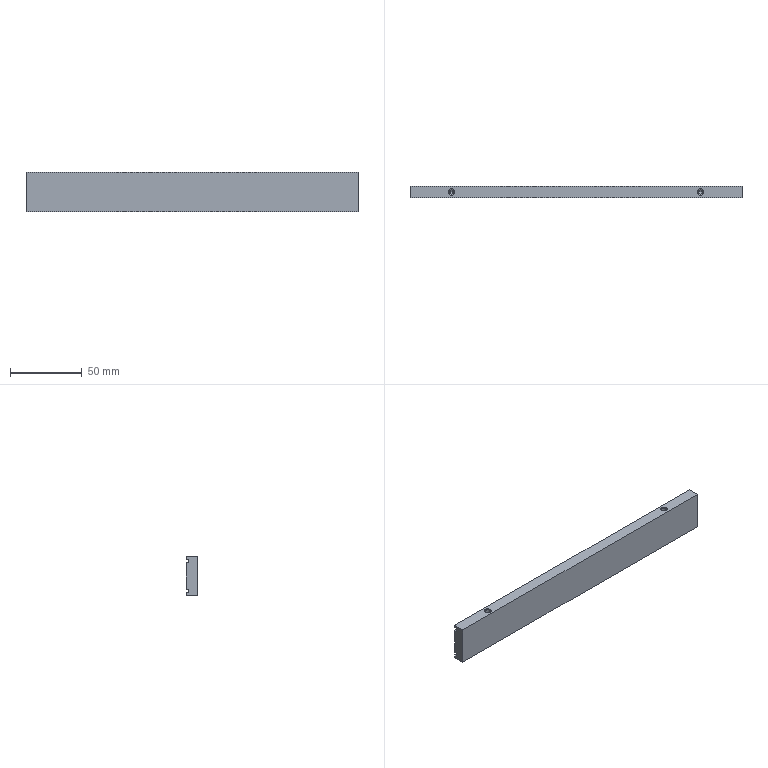Part | NX | 1 solid | 46 faces | box 232 x 8 x 27.6 mm | volume 49260 mm3 | cylinder 16 | cone 16 | plane 14 | commonest cylinder face diameters 3.3 x16
STEP:
#1=CARTESIAN_POINT('',(159.,209.7,-32.6));
#2=VERTEX_POINT('',#1);
#3=CARTESIAN_POINT('',(159.,208.2,-32.6));
#4=VERTEX_POINT('',#3);
#5=CARTESIAN_POINT('',(159.,0.,-32.6));
#6=DIRECTION('',(0.,-1.,0.));
#7=VECTOR('',#6,1000.);
#8=LINE('',#5,#7);
#9=EDGE_CURVE('',#2,#4,#8,.T.);
#10=ORIENTED_EDGE('',*,*,#9,.T.);
#11=CARTESIAN_POINT('',(391.,208.2,-32.6));
#12=VERTEX_POINT('',#11);
#13=CARTESIAN_POINT('',(0.,208.2,-32.6));
#14=DIRECTION('',(-1.,0.,0.));
#15=VECTOR('',#14,1000.);
#16=LINE('',#13,#15);
#17=EDGE_CURVE('',#12,#4,#16,.T.);
#18=ORIENTED_EDGE('',*,*,#17,.F.);
#19=CARTESIAN_POINT('',(391.,209.7,-32.6));
#20=VERTEX_POINT('',#19);
#21=CARTESIAN_POINT('',(391.,0.,-32.6));
#22=DIRECTION('',(0.,-1.,0.));
#23=VECTOR('',#22,1000.);
#24=LINE('',#21,#23);
#25=EDGE_CURVE('',#20,#12,#24,.T.);
#26=ORIENTED_EDGE('',*,*,#25,.F.);
#27=CARTESIAN_POINT('',(0.,209.7,-32.6));
#28=DIRECTION('',(1.,0.,0.));
#29=VECTOR('',#28,1000.);
#30=LINE('',#27,#29);
#31=EDGE_CURVE('',#2,#20,#30,.T.);
#32=ORIENTED_EDGE('',*,*,#31,.F.);
#33=EDGE_LOOP('',(#10,#18,#26,#32));
#34=FACE_BOUND('',#33,.T.);
#35=CARTESIAN_POINT('',(-62.051,211.112,-32.6));
#36=DIRECTION('',(0.,0.,-1.));
#37=DIRECTION('',(-1.,0.,0.));
#38=AXIS2_PLACEMENT_3D('',#35,#36,#37);
#39=PLANE('',#38);
#40=ADVANCED_FACE('',(#34),#39,.F.);
#41=CARTESIAN_POINT('',(159.,209.7,-51.4));
#42=VERTEX_POINT('',#41);
#43=CARTESIAN_POINT('',(159.,209.7,0.));
#44=DIRECTION('',(0.,0.,1.));
#45=VECTOR('',#44,1000.);
#46=LINE('',#43,#45);
#47=EDGE_CURVE('',#42,#2,#46,.T.);
#48=ORIENTED_EDGE('',*,*,#47,.T.);
#49=ORIENTED_EDGE('',*,*,#31,.T.);
#50=CARTESIAN_POINT('',(391.,209.7,-51.4));
#51=VERTEX_POINT('',#50);
#52=CARTESIAN_POINT('',(391.,209.7,0.));
#53=DIRECTION('',(0.,0.,-1.));
#54=VECTOR('',#53,1000.);
#55=LINE('',#52,#54);
#56=EDGE_CURVE('',#20,#51,#55,.T.);
#57=ORIENTED_EDGE('',*,*,#56,.T.);
#58=CARTESIAN_POINT('',(0.,209.7,-51.4));
#59=DIRECTION('',(-1.,0.,0.));
#60=VECTOR('',#59,1000.);
#61=LINE('',#58,#60);
#62=EDGE_CURVE('',#51,#42,#61,.T.);
#63=ORIENTED_EDGE('',*,*,#62,.T.);
#64=EDGE_LOOP('',(#48,#49,#57,#63));
#65=FACE_BOUND('',#64,.T.);
#66=CARTESIAN_POINT('',(652.949,209.7,-52.35));
#67=DIRECTION('',(0.,1.,0.));
#68=DIRECTION('',(1.,0.,0.));
#69=AXIS2_PLACEMENT_3D('',#66,#67,#68);
#70=PLANE('',#69);
#71=ADVANCED_FACE('',(#65),#70,.T.);
#72=ORIENTED_EDGE('',*,*,#47,.F.);
#73=CARTESIAN_POINT('',(159.,208.2,-51.4));
#74=VERTEX_POINT('',#73);
#75=CARTESIAN_POINT('',(159.,0.,-51.4));
#76=DIRECTION('',(0.,1.,0.));
#77=VECTOR('',#76,1000.);
#78=LINE('',#75,#77);
#79=EDGE_CURVE('',#74,#42,#78,.T.);
#80=ORIENTED_EDGE('',*,*,#79,.F.);
#81=CARTESIAN_POINT('',(159.,208.2,-53.6));
#82=VERTEX_POINT('',#81);
#83=CARTESIAN_POINT('',(159.,208.2,0.));
#84=DIRECTION('',(0.,0.,1.));
#85=VECTOR('',#84,1000.);
#86=LINE('',#83,#85);
#87=EDGE_CURVE('',#82,#74,#86,.T.);
#88=ORIENTED_EDGE('',*,*,#87,.F.);
#89=CARTESIAN_POINT('',(159.,209.7,-53.6));
#90=VERTEX_POINT('',#89);
#91=CARTESIAN_POINT('',(159.,0.,-53.6));
#92=DIRECTION('',(0.,-1.,0.));
#93=VECTOR('',#92,1000.);
#94=LINE('',#91,#93);
#95=EDGE_CURVE('',#90,#82,#94,.T.);
#96=ORIENTED_EDGE('',*,*,#95,.F.);
#97=CARTESIAN_POINT('',(159.,209.7,-55.8));
#98=VERTEX_POINT('',#97);
#99=CARTESIAN_POINT('',(159.,209.7,0.));
#100=DIRECTION('',(0.,0.,-1.));
#101=VECTOR('',#100,1000.);
#102=LINE('',#99,#101);
#103=EDGE_CURVE('',#90,#98,#102,.T.);
#104=ORIENTED_EDGE('',*,*,#103,.T.);
#105=CARTESIAN_POINT('',(159.,201.7,-55.8));
#106=VERTEX_POINT('',#105);
#107=CARTESIAN_POINT('',(159.,0.,-55.8));
#108=DIRECTION('',(0.,-1.,0.));
#109=VECTOR('',#108,1000.);
#110=LINE('',#107,#109);
#111=EDGE_CURVE('',#98,#106,#110,.T.);
#112=ORIENTED_EDGE('',*,*,#111,.T.);
#113=CARTESIAN_POINT('',(159.,201.7,-28.2));
#114=VERTEX_POINT('',#113);
#115=CARTESIAN_POINT('',(159.,201.7,0.));
#116=DIRECTION('',(0.,0.,1.));
#117=VECTOR('',#116,1000.);
#118=LINE('',#115,#117);
#119=EDGE_CURVE('',#106,#114,#118,.T.);
#120=ORIENTED_EDGE('',*,*,#119,.T.);
#121=CARTESIAN_POINT('',(159.,209.7,-28.2));
#122=VERTEX_POINT('',#121);
#123=CARTESIAN_POINT('',(159.,0.,-28.2));
#124=DIRECTION('',(0.,1.,0.));
#125=VECTOR('',#124,1000.);
#126=LINE('',#123,#125);
#127=EDGE_CURVE('',#114,#122,#126,.T.);
#128=ORIENTED_EDGE('',*,*,#127,.T.);
#129=CARTESIAN_POINT('',(159.,209.7,-30.4));
#130=VERTEX_POINT('',#129);
#131=CARTESIAN_POINT('',(159.,209.7,0.));
#132=DIRECTION('',(0.,0.,-1.));
#133=VECTOR('',#132,1000.);
#134=LINE('',#131,#133);
#135=EDGE_CURVE('',#122,#130,#134,.T.);
#136=ORIENTED_EDGE('',*,*,#135,.T.);
#137=CARTESIAN_POINT('',(159.,208.2,-30.4));
#138=VERTEX_POINT('',#137);
#139=CARTESIAN_POINT('',(159.,0.,-30.4));
#140=DIRECTION('',(0.,1.,0.));
#141=VECTOR('',#140,1000.);
#142=LINE('',#139,#141);
#143=EDGE_CURVE('',#138,#130,#142,.T.);
#144=ORIENTED_EDGE('',*,*,#143,.F.);
#145=CARTESIAN_POINT('',(159.,208.2,0.));
#146=DIRECTION('',(0.,0.,-1.));
#147=VECTOR('',#146,1000.);
#148=LINE('',#145,#147);
#149=EDGE_CURVE('',#138,#4,#148,.T.);
#150=ORIENTED_EDGE('',*,*,#149,.T.);
#151=ORIENTED_EDGE('',*,*,#9,.F.);
#152=EDGE_LOOP('',(#72,#80,#88,#96,#104,#112,#120,#128,#136,#144,#150,#151));
#153=FACE_BOUND('',#152,.T.);
#154=CARTESIAN_POINT('',(159.,275.752,-58.56));
#155=DIRECTION('',(1.,0.,0.));
#156=DIRECTION('',(0.,1.,0.));
#157=AXIS2_PLACEMENT_3D('',#154,#155,#156);
#158=PLANE('',#157);
#159=ADVANCED_FACE('',(#153),#158,.F.);
#160=CARTESIAN_POINT('',(391.,209.7,-30.4));
#161=VERTEX_POINT('',#160);
#162=CARTESIAN_POINT('',(391.,208.2,-30.4));
#163=VERTEX_POINT('',#162);
#164=CARTESIAN_POINT('',(391.,0.,-30.4));
#165=DIRECTION('',(0.,-1.,0.));
#166=VECTOR('',#165,1000.);
#167=LINE('',#164,#166);
#168=EDGE_CURVE('',#161,#163,#167,.T.);
#169=ORIENTED_EDGE('',*,*,#168,.T.);
#170=CARTESIAN_POINT('',(0.,208.2,-30.4));
#171=DIRECTION('',(1.,0.,0.));
#172=VECTOR('',#171,1000.);
#173=LINE('',#170,#172);
#174=EDGE_CURVE('',#138,#163,#173,.T.);
#175=ORIENTED_EDGE('',*,*,#174,.F.);
#176=ORIENTED_EDGE('',*,*,#143,.T.);
#177=CARTESIAN_POINT('',(0.,209.7,-30.4));
#178=DIRECTION('',(1.,0.,0.));
#179=VECTOR('',#178,1000.);
#180=LINE('',#177,#179);
#181=EDGE_CURVE('',#130,#161,#180,.T.);
#182=ORIENTED_EDGE('',*,*,#181,.T.);
#183=EDGE_LOOP('',(#169,#175,#176,#182));
#184=FACE_BOUND('',#183,.T.);
#185=CARTESIAN_POINT('',(-62.051,208.2,-30.4));
#186=DIRECTION('',(0.,0.,1.));
#187=DIRECTION('',(1.,0.,0.));
#188=AXIS2_PLACEMENT_3D('',#185,#186,#187);
#189=PLANE('',#188);
#190=ADVANCED_FACE('',(#184),#189,.F.);
#191=CARTESIAN_POINT('',(391.,208.2,-51.4));
#192=VERTEX_POINT('',#191);
#193=CARTESIAN_POINT('',(391.,208.2,-53.6));
#194=VERTEX_POINT('',#193);
#195=CARTESIAN_POINT('',(391.,208.2,0.));
#196=DIRECTION('',(0.,0.,-1.));
#197=VECTOR('',#196,1000.);
#198=LINE('',#195,#197);
#199=EDGE_CURVE('',#192,#194,#198,.T.);
#200=ORIENTED_EDGE('',*,*,#199,.T.);
#201=CARTESIAN_POINT('',(0.,208.2,-53.6));
#202=DIRECTION('',(-1.,0.,0.));
#203=VECTOR('',#202,1000.);
#204=LINE('',#201,#203);
#205=EDGE_CURVE('',#194,#82,#204,.T.);
#206=ORIENTED_EDGE('',*,*,#205,.T.);
#207=ORIENTED_EDGE('',*,*,#87,.T.);
#208=CARTESIAN_POINT('',(0.,208.2,-51.4));
#209=DIRECTION('',(1.,0.,0.));
#210=VECTOR('',#209,1000.);
#211=LINE('',#208,#210);
#212=EDGE_CURVE('',#74,#192,#211,.T.);
#213=ORIENTED_EDGE('',*,*,#212,.T.);
#214=EDGE_LOOP('',(#200,#206,#207,#213));
#215=FACE_BOUND('',#214,.T.);
#216=CARTESIAN_POINT('',(-62.051,208.2,-53.5));
#217=DIRECTION('',(0.,-1.,0.));
#218=DIRECTION('',(-1.,0.,0.));
#219=AXIS2_PLACEMENT_3D('',#216,#217,#218);
#220=PLANE('',#219);
#221=ADVANCED_FACE('',(#215),#220,.F.);
#222=ORIENTED_EDGE('',*,*,#95,.T.);
#223=ORIENTED_EDGE('',*,*,#205,.F.);
#224=CARTESIAN_POINT('',(391.,209.7,-53.6));
#225=VERTEX_POINT('',#224);
#226=CARTESIAN_POINT('',(391.,0.,-53.6));
#227=DIRECTION('',(0.,1.,0.));
#228=VECTOR('',#227,1000.);
#229=LINE('',#226,#228);
#230=EDGE_CURVE('',#194,#225,#229,.T.);
#231=ORIENTED_EDGE('',*,*,#230,.T.);
#232=CARTESIAN_POINT('',(0.,209.7,-53.6));
#233=DIRECTION('',(1.,0.,0.));
#234=VECTOR('',#233,1000.);
#235=LINE('',#232,#234);
#236=EDGE_CURVE('',#90,#225,#235,.T.);
#237=ORIENTED_EDGE('',*,*,#236,.F.);
#238=EDGE_LOOP('',(#222,#223,#231,#237));
#239=FACE_BOUND('',#238,.T.);
#240=CARTESIAN_POINT('',(-62.051,212.2,-53.6));
#241=DIRECTION('',(0.,0.,-1.));
#242=DIRECTION('',(-1.,0.,0.));
#243=AXIS2_PLACEMENT_3D('',#240,#241,#242);
#244=PLANE('',#243);
#245=ADVANCED_FACE('',(#239),#244,.F.);
#246=ORIENTED_EDGE('',*,*,#103,.F.);
#247=ORIENTED_EDGE('',*,*,#236,.T.);
#248=CARTESIAN_POINT('',(391.,209.7,-55.8));
#249=VERTEX_POINT('',#248);
#250=CARTESIAN_POINT('',(391.,209.7,0.));
#251=DIRECTION('',(0.,0.,1.));
#252=VECTOR('',#251,1000.);
#253=LINE('',#250,#252);
#254=EDGE_CURVE('',#249,#225,#253,.T.);
#255=ORIENTED_EDGE('',*,*,#254,.F.);
#256=CARTESIAN_POINT('',(0.,209.7,-55.8));
#257=DIRECTION('',(1.,0.,0.));
#258=VECTOR('',#257,1000.);
#259=LINE('',#256,#258);
#260=EDGE_CURVE('',#98,#249,#259,.T.);
#261=ORIENTED_EDGE('',*,*,#260,.F.);
#262=EDGE_LOOP('',(#246,#247,#255,#261));
#263=FACE_BOUND('',#262,.T.);
#264=CARTESIAN_POINT('',(652.949,209.7,-52.35));
#265=DIRECTION('',(0.,1.,0.));
#266=DIRECTION('',(1.,0.,0.));
#267=AXIS2_PLACEMENT_3D('',#264,#265,#266);
#268=PLANE('',#267);
#269=ADVANCED_FACE('',(#263),#268,.T.);
#270=CARTESIAN_POINT('',(391.,209.7,-28.2));
#271=VERTEX_POINT('',#270);
#272=CARTESIAN_POINT('',(391.,201.7,-28.2));
#273=VERTEX_POINT('',#272);
#274=CARTESIAN_POINT('',(391.,0.,-28.2));
#275=DIRECTION('',(0.,-1.,0.));
#276=VECTOR('',#275,1000.);
#277=LINE('',#274,#276);
#278=EDGE_CURVE('',#271,#273,#277,.T.);
#279=ORIENTED_EDGE('',*,*,#278,.F.);
#280=CARTESIAN_POINT('',(0.,209.7,-28.2));
#281=DIRECTION('',(-1.,0.,0.));
#282=VECTOR('',#281,1000.);
#283=LINE('',#280,#282);
#284=EDGE_CURVE('',#271,#122,#283,.T.);
#285=ORIENTED_EDGE('',*,*,#284,.T.);
#286=ORIENTED_EDGE('',*,*,#127,.F.);
#287=CARTESIAN_POINT('',(0.,201.7,-28.2));
#288=DIRECTION('',(-1.,0.,0.));
#289=VECTOR('',#288,1000.);
#290=LINE('',#287,#289);
#291=EDGE_CURVE('',#273,#114,#290,.T.);
#292=ORIENTED_EDGE('',*,*,#291,.F.);
#293=EDGE_LOOP('',(#279,#285,#286,#292));
#294=FACE_BOUND('',#293,.T.);
#295=CARTESIAN_POINT('',(185.685,205.7,-28.2));
#296=VERTEX_POINT('',#295);
#297=CARTESIAN_POINT('',(190.315,205.7,-28.2));
#298=VERTEX_POINT('',#297);
#299=CARTESIAN_POINT('',(188.,205.7,-28.2));
#300=DIRECTION('',(0.,0.,1.));
#301=DIRECTION('',(1.,0.,0.));
#302=AXIS2_PLACEMENT_3D('',#299,#300,#301);
#303=CIRCLE('',#302,2.315);
#304=EDGE_CURVE('',#296,#298,#303,.T.);
#305=ORIENTED_EDGE('',*,*,#304,.F.);
#306=CARTESIAN_POINT('',(188.,205.7,-28.2));
#307=DIRECTION('',(0.,0.,1.));
#308=DIRECTION('',(1.,0.,0.));
#309=AXIS2_PLACEMENT_3D('',#306,#307,#308);
#310=CIRCLE('',#309,2.315);
#311=EDGE_CURVE('',#298,#296,#310,.T.);
#312=ORIENTED_EDGE('',*,*,#311,.F.);
#313=EDGE_LOOP('',(#305,#312));
#314=FACE_BOUND('',#313,.T.);
#315=CARTESIAN_POINT('',(359.685,205.7,-28.2));
#316=VERTEX_POINT('',#315);
#317=CARTESIAN_POINT('',(364.315,205.7,-28.2));
#318=VERTEX_POINT('',#317);
#319=CARTESIAN_POINT('',(362.,205.7,-28.2));
#320=DIRECTION('',(0.,0.,1.));
#321=DIRECTION('',(1.,0.,0.));
#322=AXIS2_PLACEMENT_3D('',#319,#320,#321);
#323=CIRCLE('',#322,2.315);
#324=EDGE_CURVE('',#316,#318,#323,.T.);
#325=ORIENTED_EDGE('',*,*,#324,.F.);
#326=CARTESIAN_POINT('',(362.,205.7,-28.2));
#327=DIRECTION('',(0.,0.,1.));
#328=DIRECTION('',(1.,0.,0.));
#329=AXIS2_PLACEMENT_3D('',#326,#327,#328);
#330=CIRCLE('',#329,2.315);
#331=EDGE_CURVE('',#318,#316,#330,.T.);
#332=ORIENTED_EDGE('',*,*,#331,.F.);
#333=EDGE_LOOP('',(#325,#332));
#334=FACE_BOUND('',#333,.T.);
#335=CARTESIAN_POINT('',(652.949,210.2,-28.2));
#336=DIRECTION('',(0.,0.,1.));
#337=DIRECTION('',(1.,0.,0.));
#338=AXIS2_PLACEMENT_3D('',#335,#336,#337);
#339=PLANE('',#338);
#340=ADVANCED_FACE('',(#294,#314,#334),#339,.T.);
#341=CARTESIAN_POINT('',(391.,201.7,-55.8));
#342=VERTEX_POINT('',#341);
#343=CARTESIAN_POINT('',(391.,201.7,0.));
#344=DIRECTION('',(0.,0.,-1.));
#345=VECTOR('',#344,1000.);
#346=LINE('',#343,#345);
#347=EDGE_CURVE('',#273,#342,#346,.T.);
#348=ORIENTED_EDGE('',*,*,#347,.F.);
#349=ORIENTED_EDGE('',*,*,#291,.T.);
#350=ORIENTED_EDGE('',*,*,#119,.F.);
#351=CARTESIAN_POINT('',(0.,201.7,-55.8));
#352=DIRECTION('',(1.,0.,0.));
#353=VECTOR('',#352,1000.);
#354=LINE('',#351,#353);
#355=EDGE_CURVE('',#106,#342,#354,.T.);
#356=ORIENTED_EDGE('',*,*,#355,.T.);
#357=EDGE_LOOP('',(#348,#349,#350,#356));
#358=FACE_BOUND('',#357,.T.);
#359=CARTESIAN_POINT('',(652.949,201.7,-28.2));
#360=DIRECTION('',(0.,-1.,0.));
#361=DIRECTION('',(-1.,0.,0.));
#362=AXIS2_PLACEMENT_3D('',#359,#360,#361);
#363=PLANE('',#362);
#364=ADVANCED_FACE('',(#358),#363,.T.);
#365=CARTESIAN_POINT('',(391.,0.,-55.8));
#366=DIRECTION('',(0.,1.,0.));
#367=VECTOR('',#366,1000.);
#368=LINE('',#365,#367);
#369=EDGE_CURVE('',#342,#249,#368,.T.);
#370=ORIENTED_EDGE('',*,*,#369,.F.);
#371=ORIENTED_EDGE('',*,*,#355,.F.);
#372=ORIENTED_EDGE('',*,*,#111,.F.);
#373=ORIENTED_EDGE('',*,*,#260,.T.);
#374=EDGE_LOOP('',(#370,#371,#372,#373));
#375=FACE_BOUND('',#374,.T.);
#376=CARTESIAN_POINT('',(364.315,205.7,-55.8));
#377=VERTEX_POINT('',#376);
#378=CARTESIAN_POINT('',(359.685,205.7,-55.8));
#379=VERTEX_POINT('',#378);
#380=CARTESIAN_POINT('',(362.,205.7,-55.8));
#381=DIRECTION('',(0.,0.,-1.));
#382=DIRECTION('',(-1.,0.,0.));
#383=AXIS2_PLACEMENT_3D('',#380,#381,#382);
#384=CIRCLE('',#383,2.315);
#385=EDGE_CURVE('',#377,#379,#384,.T.);
#386=ORIENTED_EDGE('',*,*,#385,.F.);
#387=CARTESIAN_POINT('',(362.,205.7,-55.8));
#388=DIRECTION('',(0.,0.,-1.));
#389=DIRECTION('',(-1.,0.,0.));
#390=AXIS2_PLACEMENT_3D('',#387,#388,#389);
#391=CIRCLE('',#390,2.315);
#392=EDGE_CURVE('',#379,#377,#391,.T.);
#393=ORIENTED_EDGE('',*,*,#392,.F.);
#394=EDGE_LOOP('',(#386,#393));
#395=FACE_BOUND('',#394,.T.);
#396=CARTESIAN_POINT('',(190.315,205.7,-55.8));
#397=VERTEX_POINT('',#396);
#398=CARTESIAN_POINT('',(185.685,205.7,-55.8));
#399=VERTEX_POINT('',#398);
#400=CARTESIAN_POINT('',(188.,205.7,-55.8));
#401=DIRECTION('',(0.,0.,-1.));
#402=DIRECTION('',(-1.,0.,0.));
#403=AXIS2_PLACEMENT_3D('',#400,#401,#402);
#404=CIRCLE('',#403,2.315);
#405=EDGE_CURVE('',#397,#399,#404,.T.);
#406=ORIENTED_EDGE('',*,*,#405,.F.);
#407=CARTESIAN_POINT('',(188.,205.7,-55.8));
#408=DIRECTION('',(0.,0.,-1.));
#409=DIRECTION('',(-1.,0.,0.));
#410=AXIS2_PLACEMENT_3D('',#407,#408,#409);
#411=CIRCLE('',#410,2.315);
#412=EDGE_CURVE('',#399,#397,#411,.T.);
#413=ORIENTED_EDGE('',*,*,#412,.F.);
#414=EDGE_LOOP('',(#406,#413));
#415=FACE_BOUND('',#414,.T.);
#416=CARTESIAN_POINT('',(652.949,201.7,-55.8));
#417=DIRECTION('',(0.,0.,-1.));
#418=DIRECTION('',(-1.,0.,0.));
#419=AXIS2_PLACEMENT_3D('',#416,#417,#418);
#420=PLANE('',#419);
#421=ADVANCED_FACE('',(#375,#395,#415),#420,.T.);
#422=CARTESIAN_POINT('',(391.,209.7,0.));
#423=DIRECTION('',(0.,0.,1.));
#424=VECTOR('',#423,1000.);
#425=LINE('',#422,#424);
#426=EDGE_CURVE('',#161,#271,#425,.T.);
#427=ORIENTED_EDGE('',*,*,#426,.F.);
#428=ORIENTED_EDGE('',*,*,#181,.F.);
#429=ORIENTED_EDGE('',*,*,#135,.F.);
#430=ORIENTED_EDGE('',*,*,#284,.F.);
#431=EDGE_LOOP('',(#427,#428,#429,#430));
#432=FACE_BOUND('',#431,.T.);
#433=CARTESIAN_POINT('',(652.949,209.7,-52.35));
#434=DIRECTION('',(0.,1.,0.));
#435=DIRECTION('',(1.,0.,0.));
#436=AXIS2_PLACEMENT_3D('',#433,#434,#435);
#437=PLANE('',#436);
#438=ADVANCED_FACE('',(#432),#437,.T.);
#439=CARTESIAN_POINT('',(391.,208.2,0.));
#440=DIRECTION('',(0.,0.,1.));
#441=VECTOR('',#440,1000.);
#442=LINE('',#439,#441);
#443=EDGE_CURVE('',#12,#163,#442,.T.);
#444=ORIENTED_EDGE('',*,*,#443,.F.);
#445=ORIENTED_EDGE('',*,*,#17,.T.);
#446=ORIENTED_EDGE('',*,*,#149,.F.);
#447=ORIENTED_EDGE('',*,*,#174,.T.);
#448=EDGE_LOOP('',(#444,#445,#446,#447));
#449=FACE_BOUND('',#448,.T.);
#450=CARTESIAN_POINT('',(-62.051,208.2,-32.5));
#451=DIRECTION('',(0.,-1.,0.));
#452=DIRECTION('',(-1.,0.,0.));
#453=AXIS2_PLACEMENT_3D('',#450,#451,#452);
#454=PLANE('',#453);
#455=ADVANCED_FACE('',(#449),#454,.F.);
#456=CARTESIAN_POINT('',(391.,0.,-51.4));
#457=DIRECTION('',(0.,-1.,0.));
#458=VECTOR('',#457,1000.);
#459=LINE('',#456,#458);
#460=EDGE_CURVE('',#51,#192,#459,.T.);
#461=ORIENTED_EDGE('',*,*,#460,.T.);
#462=ORIENTED_EDGE('',*,*,#212,.F.);
#463=ORIENTED_EDGE('',*,*,#79,.T.);
#464=ORIENTED_EDGE('',*,*,#62,.F.);
#465=EDGE_LOOP('',(#461,#462,#463,#464));
#466=FACE_BOUND('',#465,.T.);
#467=CARTESIAN_POINT('',(-62.051,208.2,-51.4));
#468=DIRECTION('',(0.,0.,1.));
#469=DIRECTION('',(1.,0.,0.));
#470=AXIS2_PLACEMENT_3D('',#467,#468,#469);
#471=PLANE('',#470);
#472=ADVANCED_FACE('',(#466),#471,.F.);
#473=ORIENTED_EDGE('',*,*,#168,.F.);
#474=ORIENTED_EDGE('',*,*,#426,.T.);
#475=ORIENTED_EDGE('',*,*,#278,.T.);
#476=ORIENTED_EDGE('',*,*,#347,.T.);
#477=ORIENTED_EDGE('',*,*,#369,.T.);
#478=ORIENTED_EDGE('',*,*,#254,.T.);
#479=ORIENTED_EDGE('',*,*,#230,.F.);
#480=ORIENTED_EDGE('',*,*,#199,.F.);
#481=ORIENTED_EDGE('',*,*,#460,.F.);
#482=ORIENTED_EDGE('',*,*,#56,.F.);
#483=ORIENTED_EDGE('',*,*,#25,.T.);
#484=ORIENTED_EDGE('',*,*,#443,.T.);
#485=EDGE_LOOP('',(#473,#474,#475,#476,#477,#478,#479,#480,#481,#482,#483,#484));
#486=FACE_BOUND('',#485,.T.);
#487=CARTESIAN_POINT('',(391.,156.7,-58.56));
#488=DIRECTION('',(-1.,0.,0.));
#489=DIRECTION('',(0.,0.,1.));
#490=AXIS2_PLACEMENT_3D('',#487,#488,#489);
#491=PLANE('',#490);
#492=ADVANCED_FACE('',(#486),#491,.F.);
#493=CARTESIAN_POINT('',(186.35,205.7,-28.584));
#494=VERTEX_POINT('',#493);
#495=CARTESIAN_POINT('',(189.65,205.7,-28.584));
#496=VERTEX_POINT('',#495);
#497=CARTESIAN_POINT('',(188.,205.7,-28.584));
#498=DIRECTION('',(0.,0.,1.));
#499=DIRECTION('',(1.,0.,0.));
#500=AXIS2_PLACEMENT_3D('',#497,#498,#499);
#501=CIRCLE('',#500,1.65);
#502=EDGE_CURVE('',#494,#496,#501,.T.);
#503=ORIENTED_EDGE('',*,*,#502,.T.);
#504=CARTESIAN_POINT('',(189.65,205.7,-36.2));
#505=VERTEX_POINT('',#504);
#506=CARTESIAN_POINT('',(189.65,205.7,-28.2));
#507=DIRECTION('',(0.,0.,1.));
#508=VECTOR('',#507,1000.);
#509=LINE('',#506,#508);
#510=EDGE_CURVE('',#505,#496,#509,.T.);
#511=ORIENTED_EDGE('',*,*,#510,.F.);
#512=CARTESIAN_POINT('',(186.35,205.7,-36.2));
#513=VERTEX_POINT('',#512);
#514=CARTESIAN_POINT('',(188.,205.7,-36.2));
#515=DIRECTION('',(0.,0.,1.));
#516=DIRECTION('',(1.,0.,0.));
#517=AXIS2_PLACEMENT_3D('',#514,#515,#516);
#518=CIRCLE('',#517,1.65);
#519=EDGE_CURVE('',#513,#505,#518,.T.);
#520=ORIENTED_EDGE('',*,*,#519,.F.);
#521=CARTESIAN_POINT('',(186.35,205.7,-28.2));
#522=DIRECTION('',(0.,0.,1.));
#523=VECTOR('',#522,1000.);
#524=LINE('',#521,#523);
#525=EDGE_CURVE('',#513,#494,#524,.T.);
#526=ORIENTED_EDGE('',*,*,#525,.T.);
#527=EDGE_LOOP('',(#503,#511,#520,#526));
#528=FACE_BOUND('',#527,.T.);
#529=CARTESIAN_POINT('',(188.,205.7,-28.2));
#530=DIRECTION('',(0.,0.,1.));
#531=DIRECTION('',(1.,0.,0.));
#532=AXIS2_PLACEMENT_3D('',#529,#530,#531);
#533=CYLINDRICAL_SURFACE('',#532,1.65);
#534=ADVANCED_FACE('',(#528),#533,.F.);
#535=ORIENTED_EDGE('',*,*,#519,.T.);
#536=CARTESIAN_POINT('',(189.65,205.7,-40.4));
#537=VERTEX_POINT('',#536);
#538=CARTESIAN_POINT('',(189.65,205.7,-28.2));
#539=DIRECTION('',(0.,0.,1.));
#540=VECTOR('',#539,1000.);
#541=LINE('',#538,#540);
#542=EDGE_CURVE('',#537,#505,#541,.T.);
#543=ORIENTED_EDGE('',*,*,#542,.F.);
#544=CARTESIAN_POINT('',(186.35,205.7,-40.4));
#545=VERTEX_POINT('',#544);
#546=CARTESIAN_POINT('',(188.,205.7,-40.4));
#547=DIRECTION('',(0.,0.,1.));
#548=DIRECTION('',(1.,0.,0.));
#549=AXIS2_PLACEMENT_3D('',#546,#547,#548);
#550=CIRCLE('',#549,1.65);
#551=EDGE_CURVE('',#545,#537,#550,.T.);
#552=ORIENTED_EDGE('',*,*,#551,.F.);
#553=CARTESIAN_POINT('',(186.35,205.7,-28.2));
#554=DIRECTION('',(0.,0.,1.));
#555=VECTOR('',#554,1000.);
#556=LINE('',#553,#555);
#557=EDGE_CURVE('',#545,#513,#556,.T.);
#558=ORIENTED_EDGE('',*,*,#557,.T.);
#559=EDGE_LOOP('',(#535,#543,#552,#558));
#560=FACE_BOUND('',#559,.T.);
#561=CARTESIAN_POINT('',(188.,205.7,-28.2));
#562=DIRECTION('',(0.,0.,1.));
#563=DIRECTION('',(1.,0.,0.));
#564=AXIS2_PLACEMENT_3D('',#561,#562,#563);
#565=CYLINDRICAL_SURFACE('',#564,1.65);
#566=ADVANCED_FACE('',(#560),#565,.F.);
#567=ORIENTED_EDGE('',*,*,#551,.T.);
#568=CARTESIAN_POINT('',(188.,205.7,-41.391));
#569=VERTEX_POINT('',#568);
#570=CARTESIAN_POINT('',(189.65,205.7,-40.4));
#571=DIRECTION('',(0.8572,0.,0.515));
#572=VECTOR('',#571,1000.);
#573=LINE('',#570,#572);
#574=EDGE_CURVE('',#537,#569,#573,.F.);
#575=ORIENTED_EDGE('',*,*,#574,.T.);
#576=CARTESIAN_POINT('',(186.35,205.7,-40.4));
#577=DIRECTION('',(-0.8572,0.,0.515));
#578=VECTOR('',#577,1000.);
#579=LINE('',#576,#578);
#580=EDGE_CURVE('',#545,#569,#579,.F.);
#581=ORIENTED_EDGE('',*,*,#580,.F.);
#582=EDGE_LOOP('',(#567,#575,#581));
#583=FACE_BOUND('',#582,.T.);
#584=CARTESIAN_POINT('',(188.,205.7,-40.4));
#585=DIRECTION('',(0.,0.,1.));
#586=DIRECTION('',(1.,0.,0.));
#587=AXIS2_PLACEMENT_3D('',#584,#585,#586);
#588=CONICAL_SURFACE('',#587,1.65,1.03);
#589=ADVANCED_FACE('',(#583),#588,.F.);
#590=ORIENTED_EDGE('',*,*,#502,.F.);
#591=CARTESIAN_POINT('',(186.35,205.7,-28.584));
#592=DIRECTION('',(-0.866,0.,0.5));
#593=VECTOR('',#592,1000.);
#594=LINE('',#591,#593);
#595=EDGE_CURVE('',#494,#296,#594,.T.);
#596=ORIENTED_EDGE('',*,*,#595,.T.);
#597=ORIENTED_EDGE('',*,*,#304,.T.);
#598=CARTESIAN_POINT('',(189.65,205.7,-28.584));
#599=DIRECTION('',(0.866,0.,0.5));
#600=VECTOR('',#599,1000.);
#601=LINE('',#598,#600);
#602=EDGE_CURVE('',#496,#298,#601,.T.);
#603=ORIENTED_EDGE('',*,*,#602,.F.);
#604=EDGE_LOOP('',(#590,#596,#597,#603));
#605=FACE_BOUND('',#604,.T.);
#606=CARTESIAN_POINT('',(188.,205.7,-28.584));
#607=DIRECTION('',(0.,0.,1.));
#608=DIRECTION('',(1.,0.,0.));
#609=AXIS2_PLACEMENT_3D('',#606,#607,#608);
#610=CONICAL_SURFACE('',#609,1.65,1.047);
#611=ADVANCED_FACE('',(#605),#610,.F.);
#612=CARTESIAN_POINT('',(360.35,205.7,-28.584));
#613=VERTEX_POINT('',#612);
#614=CARTESIAN_POINT('',(363.65,205.7,-28.584));
#615=VERTEX_POINT('',#614);
#616=CARTESIAN_POINT('',(362.,205.7,-28.584));
#617=DIRECTION('',(0.,0.,1.));
#618=DIRECTION('',(1.,0.,0.));
#619=AXIS2_PLACEMENT_3D('',#616,#617,#618);
#620=CIRCLE('',#619,1.65);
#621=EDGE_CURVE('',#613,#615,#620,.T.);
#622=ORIENTED_EDGE('',*,*,#621,.T.);
#623=CARTESIAN_POINT('',(363.65,205.7,-36.2));
#624=VERTEX_POINT('',#623);
#625=CARTESIAN_POINT('',(363.65,205.7,-28.2));
#626=DIRECTION('',(0.,0.,1.));
#627=VECTOR('',#626,1000.);
#628=LINE('',#625,#627);
#629=EDGE_CURVE('',#624,#615,#628,.T.);
#630=ORIENTED_EDGE('',*,*,#629,.F.);
#631=CARTESIAN_POINT('',(360.35,205.7,-36.2));
#632=VERTEX_POINT('',#631);
#633=CARTESIAN_POINT('',(362.,205.7,-36.2));
#634=DIRECTION('',(0.,0.,1.));
#635=DIRECTION('',(1.,0.,0.));
#636=AXIS2_PLACEMENT_3D('',#633,#634,#635);
#637=CIRCLE('',#636,1.65);
#638=EDGE_CURVE('',#632,#624,#637,.T.);
#639=ORIENTED_EDGE('',*,*,#638,.F.);
#640=CARTESIAN_POINT('',(360.35,205.7,-28.2));
#641=DIRECTION('',(0.,0.,1.));
#642=VECTOR('',#641,1000.);
#643=LINE('',#640,#642);
#644=EDGE_CURVE('',#632,#613,#643,.T.);
#645=ORIENTED_EDGE('',*,*,#644,.T.);
#646=EDGE_LOOP('',(#622,#630,#639,#645));
#647=FACE_BOUND('',#646,.T.);
#648=CARTESIAN_POINT('',(362.,205.7,-28.2));
#649=DIRECTION('',(0.,0.,1.));
#650=DIRECTION('',(1.,0.,0.));
#651=AXIS2_PLACEMENT_3D('',#648,#649,#650);
#652=CYLINDRICAL_SURFACE('',#651,1.65);
#653=ADVANCED_FACE('',(#647),#652,.F.);
#654=ORIENTED_EDGE('',*,*,#638,.T.);
#655=CARTESIAN_POINT('',(363.65,205.7,-40.4));
#656=VERTEX_POINT('',#655);
#657=CARTESIAN_POINT('',(363.65,205.7,-28.2));
#658=DIRECTION('',(0.,0.,1.));
#659=VECTOR('',#658,1000.);
#660=LINE('',#657,#659);
#661=EDGE_CURVE('',#656,#624,#660,.T.);
#662=ORIENTED_EDGE('',*,*,#661,.F.);
#663=CARTESIAN_POINT('',(360.35,205.7,-40.4));
#664=VERTEX_POINT('',#663);
#665=CARTESIAN_POINT('',(362.,205.7,-40.4));
#666=DIRECTION('',(0.,0.,1.));
#667=DIRECTION('',(1.,0.,0.));
#668=AXIS2_PLACEMENT_3D('',#665,#666,#667);
#669=CIRCLE('',#668,1.65);
#670=EDGE_CURVE('',#664,#656,#669,.T.);
#671=ORIENTED_EDGE('',*,*,#670,.F.);
#672=CARTESIAN_POINT('',(360.35,205.7,-28.2));
#673=DIRECTION('',(0.,0.,1.));
#674=VECTOR('',#673,1000.);
#675=LINE('',#672,#674);
#676=EDGE_CURVE('',#664,#632,#675,.T.);
#677=ORIENTED_EDGE('',*,*,#676,.T.);
#678=EDGE_LOOP('',(#654,#662,#671,#677));
#679=FACE_BOUND('',#678,.T.);
#680=CARTESIAN_POINT('',(362.,205.7,-28.2));
#681=DIRECTION('',(0.,0.,1.));
#682=DIRECTION('',(1.,0.,0.));
#683=AXIS2_PLACEMENT_3D('',#680,#681,#682);
#684=CYLINDRICAL_SURFACE('',#683,1.65);
#685=ADVANCED_FACE('',(#679),#684,.F.);
#686=ORIENTED_EDGE('',*,*,#670,.T.);
#687=CARTESIAN_POINT('',(362.,205.7,-41.391));
#688=VERTEX_POINT('',#687);
#689=CARTESIAN_POINT('',(363.65,205.7,-40.4));
#690=DIRECTION('',(0.8572,0.,0.515));
#691=VECTOR('',#690,1000.);
#692=LINE('',#689,#691);
#693=EDGE_CURVE('',#656,#688,#692,.F.);
#694=ORIENTED_EDGE('',*,*,#693,.T.);
#695=CARTESIAN_POINT('',(360.35,205.7,-40.4));
#696=DIRECTION('',(-0.8572,0.,0.515));
#697=VECTOR('',#696,1000.);
#698=LINE('',#695,#697);
#699=EDGE_CURVE('',#664,#688,#698,.F.);
#700=ORIENTED_EDGE('',*,*,#699,.F.);
#701=EDGE_LOOP('',(#686,#694,#700));
#702=FACE_BOUND('',#701,.T.);
#703=CARTESIAN_POINT('',(362.,205.7,-40.4));
#704=DIRECTION('',(0.,0.,1.));
#705=DIRECTION('',(1.,0.,0.));
#706=AXIS2_PLACEMENT_3D('',#703,#704,#705);
#707=CONICAL_SURFACE('',#706,1.65,1.03);
#708=ADVANCED_FACE('',(#702),#707,.F.);
#709=ORIENTED_EDGE('',*,*,#621,.F.);
#710=CARTESIAN_POINT('',(360.35,205.7,-28.584));
#711=DIRECTION('',(-0.866,0.,0.5));
#712=VECTOR('',#711,1000.);
#713=LINE('',#710,#712);
#714=EDGE_CURVE('',#613,#316,#713,.T.);
#715=ORIENTED_EDGE('',*,*,#714,.T.);
#716=ORIENTED_EDGE('',*,*,#324,.T.);
#717=CARTESIAN_POINT('',(363.65,205.7,-28.584));
#718=DIRECTION('',(0.866,0.,0.5));
#719=VECTOR('',#718,1000.);
#720=LINE('',#717,#719);
#721=EDGE_CURVE('',#615,#318,#720,.T.);
#722=ORIENTED_EDGE('',*,*,#721,.F.);
#723=EDGE_LOOP('',(#709,#715,#716,#722));
#724=FACE_BOUND('',#723,.T.);
#725=CARTESIAN_POINT('',(362.,205.7,-28.584));
#726=DIRECTION('',(0.,0.,1.));
#727=DIRECTION('',(1.,0.,0.));
#728=AXIS2_PLACEMENT_3D('',#725,#726,#727);
#729=CONICAL_SURFACE('',#728,1.65,1.047);
#730=ADVANCED_FACE('',(#724),#729,.F.);
#731=CARTESIAN_POINT('',(363.65,205.7,-55.416));
#732=VERTEX_POINT('',#731);
#733=CARTESIAN_POINT('',(360.35,205.7,-55.416));
#734=VERTEX_POINT('',#733);
#735=CARTESIAN_POINT('',(362.,205.7,-55.416));
#736=DIRECTION('',(0.,0.,-1.));
#737=DIRECTION('',(-1.,0.,0.));
#738=AXIS2_PLACEMENT_3D('',#735,#736,#737);
#739=CIRCLE('',#738,1.65);
#740=EDGE_CURVE('',#732,#734,#739,.T.);
#741=ORIENTED_EDGE('',*,*,#740,.T.);
#742=CARTESIAN_POINT('',(360.35,205.7,-47.8));
#743=VERTEX_POINT('',#742);
#744=CARTESIAN_POINT('',(360.35,205.7,-55.8));
#745=DIRECTION('',(0.,0.,-1.));
#746=VECTOR('',#745,1000.);
#747=LINE('',#744,#746);
#748=EDGE_CURVE('',#734,#743,#747,.F.);
#749=ORIENTED_EDGE('',*,*,#748,.T.);
#750=CARTESIAN_POINT('',(363.65,205.7,-47.8));
#751=VERTEX_POINT('',#750);
#752=CARTESIAN_POINT('',(362.,205.7,-47.8));
#753=DIRECTION('',(0.,0.,-1.));
#754=DIRECTION('',(-1.,0.,0.));
#755=AXIS2_PLACEMENT_3D('',#752,#753,#754);
#756=CIRCLE('',#755,1.65);
#757=EDGE_CURVE('',#751,#743,#756,.T.);
#758=ORIENTED_EDGE('',*,*,#757,.F.);
#759=CARTESIAN_POINT('',(363.65,205.7,-55.8));
#760=DIRECTION('',(0.,0.,-1.));
#761=VECTOR('',#760,1000.);
#762=LINE('',#759,#761);
#763=EDGE_CURVE('',#732,#751,#762,.F.);
#764=ORIENTED_EDGE('',*,*,#763,.F.);
#765=EDGE_LOOP('',(#741,#749,#758,#764));
#766=FACE_BOUND('',#765,.T.);
#767=CARTESIAN_POINT('',(362.,205.7,-55.8));
#768=DIRECTION('',(0.,0.,-1.));
#769=DIRECTION('',(-1.,0.,0.));
#770=AXIS2_PLACEMENT_3D('',#767,#768,#769);
#771=CYLINDRICAL_SURFACE('',#770,1.65);
#772=ADVANCED_FACE('',(#766),#771,.F.);
#773=ORIENTED_EDGE('',*,*,#757,.T.);
#774=CARTESIAN_POINT('',(360.35,205.7,-43.6));
#775=VERTEX_POINT('',#774);
#776=CARTESIAN_POINT('',(360.35,205.7,-55.8));
#777=DIRECTION('',(0.,0.,-1.));
#778=VECTOR('',#777,1000.);
#779=LINE('',#776,#778);
#780=EDGE_CURVE('',#743,#775,#779,.F.);
#781=ORIENTED_EDGE('',*,*,#780,.T.);
#782=CARTESIAN_POINT('',(363.65,205.7,-43.6));
#783=VERTEX_POINT('',#782);
#784=CARTESIAN_POINT('',(362.,205.7,-43.6));
#785=DIRECTION('',(0.,0.,-1.));
#786=DIRECTION('',(-1.,0.,0.));
#787=AXIS2_PLACEMENT_3D('',#784,#785,#786);
#788=CIRCLE('',#787,1.65);
#789=EDGE_CURVE('',#783,#775,#788,.T.);
#790=ORIENTED_EDGE('',*,*,#789,.F.);
#791=CARTESIAN_POINT('',(363.65,205.7,-55.8));
#792=DIRECTION('',(0.,0.,-1.));
#793=VECTOR('',#792,1000.);
#794=LINE('',#791,#793);
#795=EDGE_CURVE('',#751,#783,#794,.F.);
#796=ORIENTED_EDGE('',*,*,#795,.F.);
#797=EDGE_LOOP('',(#773,#781,#790,#796));
#798=FACE_BOUND('',#797,.T.);
#799=CARTESIAN_POINT('',(362.,205.7,-55.8));
#800=DIRECTION('',(0.,0.,-1.));
#801=DIRECTION('',(-1.,0.,0.));
#802=AXIS2_PLACEMENT_3D('',#799,#800,#801);
#803=CYLINDRICAL_SURFACE('',#802,1.65);
#804=ADVANCED_FACE('',(#798),#803,.F.);
#805=ORIENTED_EDGE('',*,*,#789,.T.);
#806=CARTESIAN_POINT('',(362.,205.7,-42.609));
#807=VERTEX_POINT('',#806);
#808=CARTESIAN_POINT('',(360.35,205.7,-43.6));
#809=DIRECTION('',(-0.8572,0.,-0.515));
#810=VECTOR('',#809,1000.);
#811=LINE('',#808,#810);
#812=EDGE_CURVE('',#807,#775,#811,.T.);
#813=ORIENTED_EDGE('',*,*,#812,.F.);
#814=CARTESIAN_POINT('',(363.65,205.7,-43.6));
#815=DIRECTION('',(0.8572,0.,-0.515));
#816=VECTOR('',#815,1000.);
#817=LINE('',#814,#816);
#818=EDGE_CURVE('',#807,#783,#817,.T.);
#819=ORIENTED_EDGE('',*,*,#818,.T.);
#820=EDGE_LOOP('',(#805,#813,#819));
#821=FACE_BOUND('',#820,.T.);
#822=CARTESIAN_POINT('',(362.,205.7,-43.6));
#823=DIRECTION('',(0.,0.,-1.));
#824=DIRECTION('',(-1.,0.,0.));
#825=AXIS2_PLACEMENT_3D('',#822,#823,#824);
#826=CONICAL_SURFACE('',#825,1.65,1.03);
#827=ADVANCED_FACE('',(#821),#826,.F.);
#828=ORIENTED_EDGE('',*,*,#740,.F.);
#829=CARTESIAN_POINT('',(363.65,205.7,-55.416));
#830=DIRECTION('',(0.866,0.,-0.5));
#831=VECTOR('',#830,1000.);
#832=LINE('',#829,#831);
#833=EDGE_CURVE('',#377,#732,#832,.F.);
#834=ORIENTED_EDGE('',*,*,#833,.F.);
#835=ORIENTED_EDGE('',*,*,#385,.T.);
#836=CARTESIAN_POINT('',(360.35,205.7,-55.416));
#837=DIRECTION('',(-0.866,0.,-0.5));
#838=VECTOR('',#837,1000.);
#839=LINE('',#836,#838);
#840=EDGE_CURVE('',#379,#734,#839,.F.);
#841=ORIENTED_EDGE('',*,*,#840,.T.);
#842=EDGE_LOOP('',(#828,#834,#835,#841));
#843=FACE_BOUND('',#842,.T.);
#844=CARTESIAN_POINT('',(362.,205.7,-55.416));
#845=DIRECTION('',(0.,0.,-1.));
#846=DIRECTION('',(-1.,0.,0.));
#847=AXIS2_PLACEMENT_3D('',#844,#845,#846);
#848=CONICAL_SURFACE('',#847,1.65,1.047);
#849=ADVANCED_FACE('',(#843),#848,.F.);
#850=CARTESIAN_POINT('',(189.65,205.7,-55.416));
#851=VERTEX_POINT('',#850);
#852=CARTESIAN_POINT('',(186.35,205.7,-55.416));
#853=VERTEX_POINT('',#852);
#854=CARTESIAN_POINT('',(188.,205.7,-55.416));
#855=DIRECTION('',(0.,0.,-1.));
#856=DIRECTION('',(-1.,0.,0.));
#857=AXIS2_PLACEMENT_3D('',#854,#855,#856);
#858=CIRCLE('',#857,1.65);
#859=EDGE_CURVE('',#851,#853,#858,.T.);
#860=ORIENTED_EDGE('',*,*,#859,.T.);
#861=CARTESIAN_POINT('',(186.35,205.7,-47.8));
#862=VERTEX_POINT('',#861);
#863=CARTESIAN_POINT('',(186.35,205.7,-55.8));
#864=DIRECTION('',(0.,0.,-1.));
#865=VECTOR('',#864,1000.);
#866=LINE('',#863,#865);
#867=EDGE_CURVE('',#853,#862,#866,.F.);
#868=ORIENTED_EDGE('',*,*,#867,.T.);
#869=CARTESIAN_POINT('',(189.65,205.7,-47.8));
#870=VERTEX_POINT('',#869);
#871=CARTESIAN_POINT('',(188.,205.7,-47.8));
#872=DIRECTION('',(0.,0.,-1.));
#873=DIRECTION('',(-1.,0.,0.));
#874=AXIS2_PLACEMENT_3D('',#871,#872,#873);
#875=CIRCLE('',#874,1.65);
#876=EDGE_CURVE('',#870,#862,#875,.T.);
#877=ORIENTED_EDGE('',*,*,#876,.F.);
#878=CARTESIAN_POINT('',(189.65,205.7,-55.8));
#879=DIRECTION('',(0.,0.,-1.));
#880=VECTOR('',#879,1000.);
#881=LINE('',#878,#880);
#882=EDGE_CURVE('',#851,#870,#881,.F.);
#883=ORIENTED_EDGE('',*,*,#882,.F.);
#884=EDGE_LOOP('',(#860,#868,#877,#883));
#885=FACE_BOUND('',#884,.T.);
#886=CARTESIAN_POINT('',(188.,205.7,-55.8));
#887=DIRECTION('',(0.,0.,-1.));
#888=DIRECTION('',(-1.,0.,0.));
#889=AXIS2_PLACEMENT_3D('',#886,#887,#888);
#890=CYLINDRICAL_SURFACE('',#889,1.65);
#891=ADVANCED_FACE('',(#885),#890,.F.);
#892=ORIENTED_EDGE('',*,*,#876,.T.);
#893=CARTESIAN_POINT('',(186.35,205.7,-43.6));
#894=VERTEX_POINT('',#893);
#895=CARTESIAN_POINT('',(186.35,205.7,-55.8));
#896=DIRECTION('',(0.,0.,-1.));
#897=VECTOR('',#896,1000.);
#898=LINE('',#895,#897);
#899=EDGE_CURVE('',#862,#894,#898,.F.);
#900=ORIENTED_EDGE('',*,*,#899,.T.);
#901=CARTESIAN_POINT('',(189.65,205.7,-43.6));
#902=VERTEX_POINT('',#901);
#903=CARTESIAN_POINT('',(188.,205.7,-43.6));
#904=DIRECTION('',(0.,0.,-1.));
#905=DIRECTION('',(-1.,0.,0.));
#906=AXIS2_PLACEMENT_3D('',#903,#904,#905);
#907=CIRCLE('',#906,1.65);
#908=EDGE_CURVE('',#902,#894,#907,.T.);
#909=ORIENTED_EDGE('',*,*,#908,.F.);
#910=CARTESIAN_POINT('',(189.65,205.7,-55.8));
#911=DIRECTION('',(0.,0.,-1.));
#912=VECTOR('',#911,1000.);
#913=LINE('',#910,#912);
#914=EDGE_CURVE('',#870,#902,#913,.F.);
#915=ORIENTED_EDGE('',*,*,#914,.F.);
#916=EDGE_LOOP('',(#892,#900,#909,#915));
#917=FACE_BOUND('',#916,.T.);
#918=CARTESIAN_POINT('',(188.,205.7,-55.8));
#919=DIRECTION('',(0.,0.,-1.));
#920=DIRECTION('',(-1.,0.,0.));
#921=AXIS2_PLACEMENT_3D('',#918,#919,#920);
#922=CYLINDRICAL_SURFACE('',#921,1.65);
#923=ADVANCED_FACE('',(#917),#922,.F.);
#924=ORIENTED_EDGE('',*,*,#908,.T.);
#925=CARTESIAN_POINT('',(188.,205.7,-42.609));
#926=VERTEX_POINT('',#925);
#927=CARTESIAN_POINT('',(186.35,205.7,-43.6));
#928=DIRECTION('',(-0.8572,0.,-0.515));
#929=VECTOR('',#928,1000.);
#930=LINE('',#927,#929);
#931=EDGE_CURVE('',#926,#894,#930,.T.);
#932=ORIENTED_EDGE('',*,*,#931,.F.);
#933=CARTESIAN_POINT('',(189.65,205.7,-43.6));
#934=DIRECTION('',(0.8572,0.,-0.515));
#935=VECTOR('',#934,1000.);
#936=LINE('',#933,#935);
#937=EDGE_CURVE('',#926,#902,#936,.T.);
#938=ORIENTED_EDGE('',*,*,#937,.T.);
#939=EDGE_LOOP('',(#924,#932,#938));
#940=FACE_BOUND('',#939,.T.);
#941=CARTESIAN_POINT('',(188.,205.7,-43.6));
#942=DIRECTION('',(0.,0.,-1.));
#943=DIRECTION('',(-1.,0.,0.));
#944=AXIS2_PLACEMENT_3D('',#941,#942,#943);
#945=CONICAL_SURFACE('',#944,1.65,1.03);
#946=ADVANCED_FACE('',(#940),#945,.F.);
#947=ORIENTED_EDGE('',*,*,#859,.F.);
#948=CARTESIAN_POINT('',(189.65,205.7,-55.416));
#949=DIRECTION('',(0.866,0.,-0.5));
#950=VECTOR('',#949,1000.);
#951=LINE('',#948,#950);
#952=EDGE_CURVE('',#397,#851,#951,.F.);
#953=ORIENTED_EDGE('',*,*,#952,.F.);
#954=ORIENTED_EDGE('',*,*,#405,.T.);
#955=CARTESIAN_POINT('',(186.35,205.7,-55.416));
#956=DIRECTION('',(-0.866,0.,-0.5));
#957=VECTOR('',#956,1000.);
#958=LINE('',#955,#957);
#959=EDGE_CURVE('',#399,#853,#958,.F.);
#960=ORIENTED_EDGE('',*,*,#959,.T.);
#961=EDGE_LOOP('',(#947,#953,#954,#960));
#962=FACE_BOUND('',#961,.T.);
#963=CARTESIAN_POINT('',(188.,205.7,-55.416));
#964=DIRECTION('',(0.,0.,-1.));
#965=DIRECTION('',(-1.,0.,0.));
#966=AXIS2_PLACEMENT_3D('',#963,#964,#965);
#967=CONICAL_SURFACE('',#966,1.65,1.047);
#968=ADVANCED_FACE('',(#962),#967,.F.);
#969=ORIENTED_EDGE('',*,*,#867,.F.);
#970=CARTESIAN_POINT('',(188.,205.7,-55.416));
#971=DIRECTION('',(0.,0.,-1.));
#972=DIRECTION('',(-1.,0.,0.));
#973=AXIS2_PLACEMENT_3D('',#970,#971,#972);
#974=CIRCLE('',#973,1.65);
#975=EDGE_CURVE('',#853,#851,#974,.T.);
#976=ORIENTED_EDGE('',*,*,#975,.T.);
#977=ORIENTED_EDGE('',*,*,#882,.T.);
#978=CARTESIAN_POINT('',(188.,205.7,-47.8));
#979=DIRECTION('',(0.,0.,-1.));
#980=DIRECTION('',(-1.,0.,0.));
#981=AXIS2_PLACEMENT_3D('',#978,#979,#980);
#982=CIRCLE('',#981,1.65);
#983=EDGE_CURVE('',#862,#870,#982,.T.);
#984=ORIENTED_EDGE('',*,*,#983,.F.);
#985=EDGE_LOOP('',(#969,#976,#977,#984));
#986=FACE_BOUND('',#985,.T.);
#987=CARTESIAN_POINT('',(188.,205.7,-55.8));
#988=DIRECTION('',(0.,0.,-1.));
#989=DIRECTION('',(-1.,0.,0.));
#990=AXIS2_PLACEMENT_3D('',#987,#988,#989);
#991=CYLINDRICAL_SURFACE('',#990,1.65);
#992=ADVANCED_FACE('',(#986),#991,.F.);
#993=ORIENTED_EDGE('',*,*,#780,.F.);
#994=CARTESIAN_POINT('',(362.,205.7,-47.8));
#995=DIRECTION('',(0.,0.,-1.));
#996=DIRECTION('',(-1.,0.,0.));
#997=AXIS2_PLACEMENT_3D('',#994,#995,#996);
#998=CIRCLE('',#997,1.65);
#999=EDGE_CURVE('',#743,#751,#998,.T.);
#1000=ORIENTED_EDGE('',*,*,#999,.T.);
#1001=ORIENTED_EDGE('',*,*,#795,.T.);
#1002=CARTESIAN_POINT('',(362.,205.7,-43.6));
#1003=DIRECTION('',(0.,0.,-1.));
#1004=DIRECTION('',(-1.,0.,0.));
#1005=AXIS2_PLACEMENT_3D('',#1002,#1003,#1004);
#1006=CIRCLE('',#1005,1.65);
#1007=EDGE_CURVE('',#775,#783,#1006,.T.);
#1008=ORIENTED_EDGE('',*,*,#1007,.F.);
#1009=EDGE_LOOP('',(#993,#1000,#1001,#1008));
#1010=FACE_BOUND('',#1009,.T.);
#1011=CARTESIAN_POINT('',(362.,205.7,-55.8));
#1012=DIRECTION('',(0.,0.,-1.));
#1013=DIRECTION('',(-1.,0.,0.));
#1014=AXIS2_PLACEMENT_3D('',#1011,#1012,#1013);
#1015=CYLINDRICAL_SURFACE('',#1014,1.65);
#1016=ADVANCED_FACE('',(#1010),#1015,.F.);
#1017=ORIENTED_EDGE('',*,*,#629,.T.);
#1018=CARTESIAN_POINT('',(362.,205.7,-28.584));
#1019=DIRECTION('',(0.,0.,1.));
#1020=DIRECTION('',(1.,0.,0.));
#1021=AXIS2_PLACEMENT_3D('',#1018,#1019,#1020);
#1022=CIRCLE('',#1021,1.65);
#1023=EDGE_CURVE('',#615,#613,#1022,.T.);
#1024=ORIENTED_EDGE('',*,*,#1023,.T.);
#1025=ORIENTED_EDGE('',*,*,#644,.F.);
#1026=CARTESIAN_POINT('',(362.,205.7,-36.2));
#1027=DIRECTION('',(0.,0.,1.));
#1028=DIRECTION('',(1.,0.,0.));
#1029=AXIS2_PLACEMENT_3D('',#1026,#1027,#1028);
#1030=CIRCLE('',#1029,1.65);
#1031=EDGE_CURVE('',#624,#632,#1030,.T.);
#1032=ORIENTED_EDGE('',*,*,#1031,.F.);
#1033=EDGE_LOOP('',(#1017,#1024,#1025,#1032));
#1034=FACE_BOUND('',#1033,.T.);
#1035=CARTESIAN_POINT('',(362.,205.7,-28.2));
#1036=DIRECTION('',(0.,0.,1.));
#1037=DIRECTION('',(1.,0.,0.));
#1038=AXIS2_PLACEMENT_3D('',#1035,#1036,#1037);
#1039=CYLINDRICAL_SURFACE('',#1038,1.65);
#1040=ADVANCED_FACE('',(#1034),#1039,.F.);
#1041=ORIENTED_EDGE('',*,*,#580,.T.);
#1042=ORIENTED_EDGE('',*,*,#574,.F.);
#1043=CARTESIAN_POINT('',(188.,205.7,-40.4));
#1044=DIRECTION('',(0.,0.,1.));
#1045=DIRECTION('',(1.,0.,0.));
#1046=AXIS2_PLACEMENT_3D('',#1043,#1044,#1045);
#1047=CIRCLE('',#1046,1.65);
#1048=EDGE_CURVE('',#537,#545,#1047,.T.);
#1049=ORIENTED_EDGE('',*,*,#1048,.T.);
#1050=EDGE_LOOP('',(#1041,#1042,#1049));
#1051=FACE_BOUND('',#1050,.T.);
#1052=CARTESIAN_POINT('',(188.,205.7,-40.4));
#1053=DIRECTION('',(0.,0.,1.));
#1054=DIRECTION('',(1.,0.,0.));
#1055=AXIS2_PLACEMENT_3D('',#1052,#1053,#1054);
#1056=CONICAL_SURFACE('',#1055,1.65,1.03);
#1057=ADVANCED_FACE('',(#1051),#1056,.F.);
#1058=ORIENTED_EDGE('',*,*,#899,.F.);
#1059=ORIENTED_EDGE('',*,*,#983,.T.);
#1060=ORIENTED_EDGE('',*,*,#914,.T.);
#1061=CARTESIAN_POINT('',(188.,205.7,-43.6));
#1062=DIRECTION('',(0.,0.,-1.));
#1063=DIRECTION('',(-1.,0.,0.));
#1064=AXIS2_PLACEMENT_3D('',#1061,#1062,#1063);
#1065=CIRCLE('',#1064,1.65);
#1066=EDGE_CURVE('',#894,#902,#1065,.T.);
#1067=ORIENTED_EDGE('',*,*,#1066,.F.);
#1068=EDGE_LOOP('',(#1058,#1059,#1060,#1067));
#1069=FACE_BOUND('',#1068,.T.);
#1070=CARTESIAN_POINT('',(188.,205.7,-55.8));
#1071=DIRECTION('',(0.,0.,-1.));
#1072=DIRECTION('',(-1.,0.,0.));
#1073=AXIS2_PLACEMENT_3D('',#1070,#1071,#1072);
#1074=CYLINDRICAL_SURFACE('',#1073,1.65);
#1075=ADVANCED_FACE('',(#1069),#1074,.F.);
#1076=ORIENTED_EDGE('',*,*,#602,.T.);
#1077=ORIENTED_EDGE('',*,*,#311,.T.);
#1078=ORIENTED_EDGE('',*,*,#595,.F.);
#1079=CARTESIAN_POINT('',(188.,205.7,-28.584));
#1080=DIRECTION('',(0.,0.,1.));
#1081=DIRECTION('',(1.,0.,0.));
#1082=AXIS2_PLACEMENT_3D('',#1079,#1080,#1081);
#1083=CIRCLE('',#1082,1.65);
#1084=EDGE_CURVE('',#496,#494,#1083,.T.);
#1085=ORIENTED_EDGE('',*,*,#1084,.F.);
#1086=EDGE_LOOP('',(#1076,#1077,#1078,#1085));
#1087=FACE_BOUND('',#1086,.T.);
#1088=CARTESIAN_POINT('',(188.,205.7,-28.584));
#1089=DIRECTION('',(0.,0.,1.));
#1090=DIRECTION('',(1.,0.,0.));
#1091=AXIS2_PLACEMENT_3D('',#1088,#1089,#1090);
#1092=CONICAL_SURFACE('',#1091,1.65,1.047);
#1093=ADVANCED_FACE('',(#1087),#1092,.F.);
#1094=ORIENTED_EDGE('',*,*,#818,.F.);
#1095=ORIENTED_EDGE('',*,*,#812,.T.);
#1096=ORIENTED_EDGE('',*,*,#1007,.T.);
#1097=EDGE_LOOP('',(#1094,#1095,#1096));
#1098=FACE_BOUND('',#1097,.T.);
#1099=CARTESIAN_POINT('',(362.,205.7,-43.6));
#1100=DIRECTION('',(0.,0.,-1.));
#1101=DIRECTION('',(-1.,0.,0.));
#1102=AXIS2_PLACEMENT_3D('',#1099,#1100,#1101);
#1103=CONICAL_SURFACE('',#1102,1.65,1.03);
#1104=ADVANCED_FACE('',(#1098),#1103,.F.);
#1105=ORIENTED_EDGE('',*,*,#840,.F.);
#1106=ORIENTED_EDGE('',*,*,#392,.T.);
#1107=ORIENTED_EDGE('',*,*,#833,.T.);
#1108=CARTESIAN_POINT('',(362.,205.7,-55.416));
#1109=DIRECTION('',(0.,0.,-1.));
#1110=DIRECTION('',(-1.,0.,0.));
#1111=AXIS2_PLACEMENT_3D('',#1108,#1109,#1110);
#1112=CIRCLE('',#1111,1.65);
#1113=EDGE_CURVE('',#734,#732,#1112,.T.);
#1114=ORIENTED_EDGE('',*,*,#1113,.F.);
#1115=EDGE_LOOP('',(#1105,#1106,#1107,#1114));
#1116=FACE_BOUND('',#1115,.T.);
#1117=CARTESIAN_POINT('',(362.,205.7,-55.416));
#1118=DIRECTION('',(0.,0.,-1.));
#1119=DIRECTION('',(-1.,0.,0.));
#1120=AXIS2_PLACEMENT_3D('',#1117,#1118,#1119);
#1121=CONICAL_SURFACE('',#1120,1.65,1.047);
#1122=ADVANCED_FACE('',(#1116),#1121,.F.);
#1123=ORIENTED_EDGE('',*,*,#661,.T.);
#1124=ORIENTED_EDGE('',*,*,#1031,.T.);
#1125=ORIENTED_EDGE('',*,*,#676,.F.);
#1126=CARTESIAN_POINT('',(362.,205.7,-40.4));
#1127=DIRECTION('',(0.,0.,1.));
#1128=DIRECTION('',(1.,0.,0.));
#1129=AXIS2_PLACEMENT_3D('',#1126,#1127,#1128);
#1130=CIRCLE('',#1129,1.65);
#1131=EDGE_CURVE('',#656,#664,#1130,.T.);
#1132=ORIENTED_EDGE('',*,*,#1131,.F.);
#1133=EDGE_LOOP('',(#1123,#1124,#1125,#1132));
#1134=FACE_BOUND('',#1133,.T.);
#1135=CARTESIAN_POINT('',(362.,205.7,-28.2));
#1136=DIRECTION('',(0.,0.,1.));
#1137=DIRECTION('',(1.,0.,0.));
#1138=AXIS2_PLACEMENT_3D('',#1135,#1136,#1137);
#1139=CYLINDRICAL_SURFACE('',#1138,1.65);
#1140=ADVANCED_FACE('',(#1134),#1139,.F.);
#1141=ORIENTED_EDGE('',*,*,#937,.F.);
#1142=ORIENTED_EDGE('',*,*,#931,.T.);
#1143=ORIENTED_EDGE('',*,*,#1066,.T.);
#1144=EDGE_LOOP('',(#1141,#1142,#1143));
#1145=FACE_BOUND('',#1144,.T.);
#1146=CARTESIAN_POINT('',(188.,205.7,-43.6));
#1147=DIRECTION('',(0.,0.,-1.));
#1148=DIRECTION('',(-1.,0.,0.));
#1149=AXIS2_PLACEMENT_3D('',#1146,#1147,#1148);
#1150=CONICAL_SURFACE('',#1149,1.65,1.03);
#1151=ADVANCED_FACE('',(#1145),#1150,.F.);
#1152=ORIENTED_EDGE('',*,*,#510,.T.);
#1153=ORIENTED_EDGE('',*,*,#1084,.T.);
#1154=ORIENTED_EDGE('',*,*,#525,.F.);
#1155=CARTESIAN_POINT('',(188.,205.7,-36.2));
#1156=DIRECTION('',(0.,0.,1.));
#1157=DIRECTION('',(1.,0.,0.));
#1158=AXIS2_PLACEMENT_3D('',#1155,#1156,#1157);
#1159=CIRCLE('',#1158,1.65);
#1160=EDGE_CURVE('',#505,#513,#1159,.T.);
#1161=ORIENTED_EDGE('',*,*,#1160,.F.);
#1162=EDGE_LOOP('',(#1152,#1153,#1154,#1161));
#1163=FACE_BOUND('',#1162,.T.);
#1164=CARTESIAN_POINT('',(188.,205.7,-28.2));
#1165=DIRECTION('',(0.,0.,1.));
#1166=DIRECTION('',(1.,0.,0.));
#1167=AXIS2_PLACEMENT_3D('',#1164,#1165,#1166);
#1168=CYLINDRICAL_SURFACE('',#1167,1.65);
#1169=ADVANCED_FACE('',(#1163),#1168,.F.);
#1170=ORIENTED_EDGE('',*,*,#959,.F.);
#1171=ORIENTED_EDGE('',*,*,#412,.T.);
#1172=ORIENTED_EDGE('',*,*,#952,.T.);
#1173=ORIENTED_EDGE('',*,*,#975,.F.);
#1174=EDGE_LOOP('',(#1170,#1171,#1172,#1173));
#1175=FACE_BOUND('',#1174,.T.);
#1176=CARTESIAN_POINT('',(188.,205.7,-55.416));
#1177=DIRECTION('',(0.,0.,-1.));
#1178=DIRECTION('',(-1.,0.,0.));
#1179=AXIS2_PLACEMENT_3D('',#1176,#1177,#1178);
#1180=CONICAL_SURFACE('',#1179,1.65,1.047);
#1181=ADVANCED_FACE('',(#1175),#1180,.F.);
#1182=ORIENTED_EDGE('',*,*,#748,.F.);
#1183=ORIENTED_EDGE('',*,*,#1113,.T.);
#1184=ORIENTED_EDGE('',*,*,#763,.T.);
#1185=ORIENTED_EDGE('',*,*,#999,.F.);
#1186=EDGE_LOOP('',(#1182,#1183,#1184,#1185));
#1187=FACE_BOUND('',#1186,.T.);
#1188=CARTESIAN_POINT('',(362.,205.7,-55.8));
#1189=DIRECTION('',(0.,0.,-1.));
#1190=DIRECTION('',(-1.,0.,0.));
#1191=AXIS2_PLACEMENT_3D('',#1188,#1189,#1190);
#1192=CYLINDRICAL_SURFACE('',#1191,1.65);
#1193=ADVANCED_FACE('',(#1187),#1192,.F.);
#1194=ORIENTED_EDGE('',*,*,#699,.T.);
#1195=ORIENTED_EDGE('',*,*,#693,.F.);
#1196=ORIENTED_EDGE('',*,*,#1131,.T.);
#1197=EDGE_LOOP('',(#1194,#1195,#1196));
#1198=FACE_BOUND('',#1197,.T.);
#1199=CARTESIAN_POINT('',(362.,205.7,-40.4));
#1200=DIRECTION('',(0.,0.,1.));
#1201=DIRECTION('',(1.,0.,0.));
#1202=AXIS2_PLACEMENT_3D('',#1199,#1200,#1201);
#1203=CONICAL_SURFACE('',#1202,1.65,1.03);
#1204=ADVANCED_FACE('',(#1198),#1203,.F.);
#1205=ORIENTED_EDGE('',*,*,#721,.T.);
#1206=ORIENTED_EDGE('',*,*,#331,.T.);
#1207=ORIENTED_EDGE('',*,*,#714,.F.);
#1208=ORIENTED_EDGE('',*,*,#1023,.F.);
#1209=EDGE_LOOP('',(#1205,#1206,#1207,#1208));
#1210=FACE_BOUND('',#1209,.T.);
#1211=CARTESIAN_POINT('',(362.,205.7,-28.584));
#1212=DIRECTION('',(0.,0.,1.));
#1213=DIRECTION('',(1.,0.,0.));
#1214=AXIS2_PLACEMENT_3D('',#1211,#1212,#1213);
#1215=CONICAL_SURFACE('',#1214,1.65,1.047);
#1216=ADVANCED_FACE('',(#1210),#1215,.F.);
#1217=ORIENTED_EDGE('',*,*,#542,.T.);
#1218=ORIENTED_EDGE('',*,*,#1160,.T.);
#1219=ORIENTED_EDGE('',*,*,#557,.F.);
#1220=ORIENTED_EDGE('',*,*,#1048,.F.);
#1221=EDGE_LOOP('',(#1217,#1218,#1219,#1220));
#1222=FACE_BOUND('',#1221,.T.);
#1223=CARTESIAN_POINT('',(188.,205.7,-28.2));
#1224=DIRECTION('',(0.,0.,1.));
#1225=DIRECTION('',(1.,0.,0.));
#1226=AXIS2_PLACEMENT_3D('',#1223,#1224,#1225);
#1227=CYLINDRICAL_SURFACE('',#1226,1.65);
#1228=ADVANCED_FACE('',(#1222),#1227,.F.);
#1229=CLOSED_SHELL('',(#40,#71,#159,#190,#221,#245,#269,#340,#364,#421,#438,#455,#472,#492,#534,#566,#589,#611,#653,#685,#708,#730,#772,#804,#827,#849,#891,#923,#946,#968,#992,#1016,#1040,#1057,#1075,#1093,#1104,#1122,#1140,#1151,#1169,#1181,#1193,#1204,#1216,#1228));
#1230=MANIFOLD_SOLID_BREP('',#1229);
#1231=(LENGTH_UNIT()NAMED_UNIT(*)SI_UNIT(.MILLI.,.METRE.));
#1232=UNCERTAINTY_MEASURE_WITH_UNIT(LENGTH_MEASURE(0.00001),#1231,'','');
#1233=(NAMED_UNIT(*)PLANE_ANGLE_UNIT()SI_UNIT($,.RADIAN.));
#1234=(NAMED_UNIT(*)SI_UNIT($,.STERADIAN.)SOLID_ANGLE_UNIT());
#1235=(GEOMETRIC_REPRESENTATION_CONTEXT(3)GLOBAL_UNCERTAINTY_ASSIGNED_CONTEXT((#1232))GLOBAL_UNIT_ASSIGNED_CONTEXT((#1231,#1233,#1234))REPRESENTATION_CONTEXT('',''));
#1236=ADVANCED_BREP_SHAPE_REPRESENTATION('',(#1230),#1235);